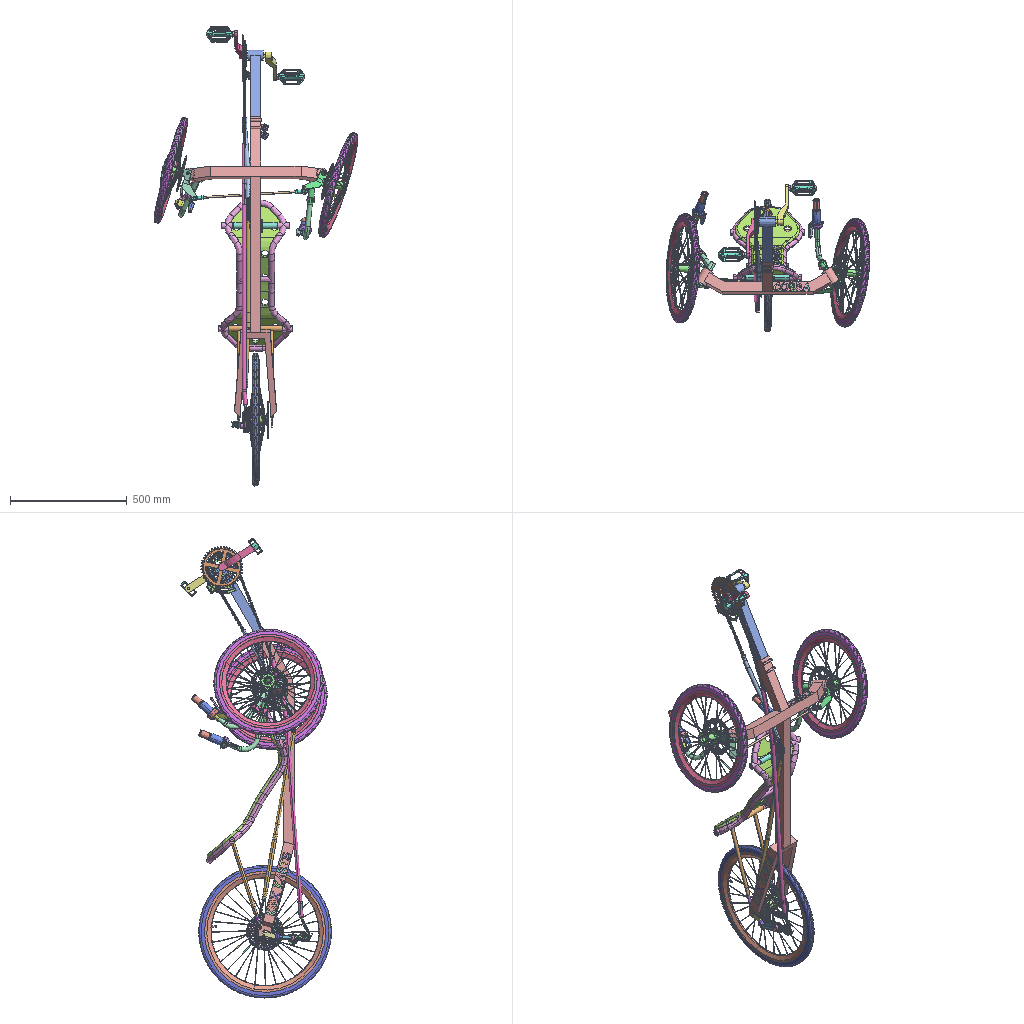Assembly | STEP file | 85 different items | 198 placed | box 873 x 646 x 1971 mm
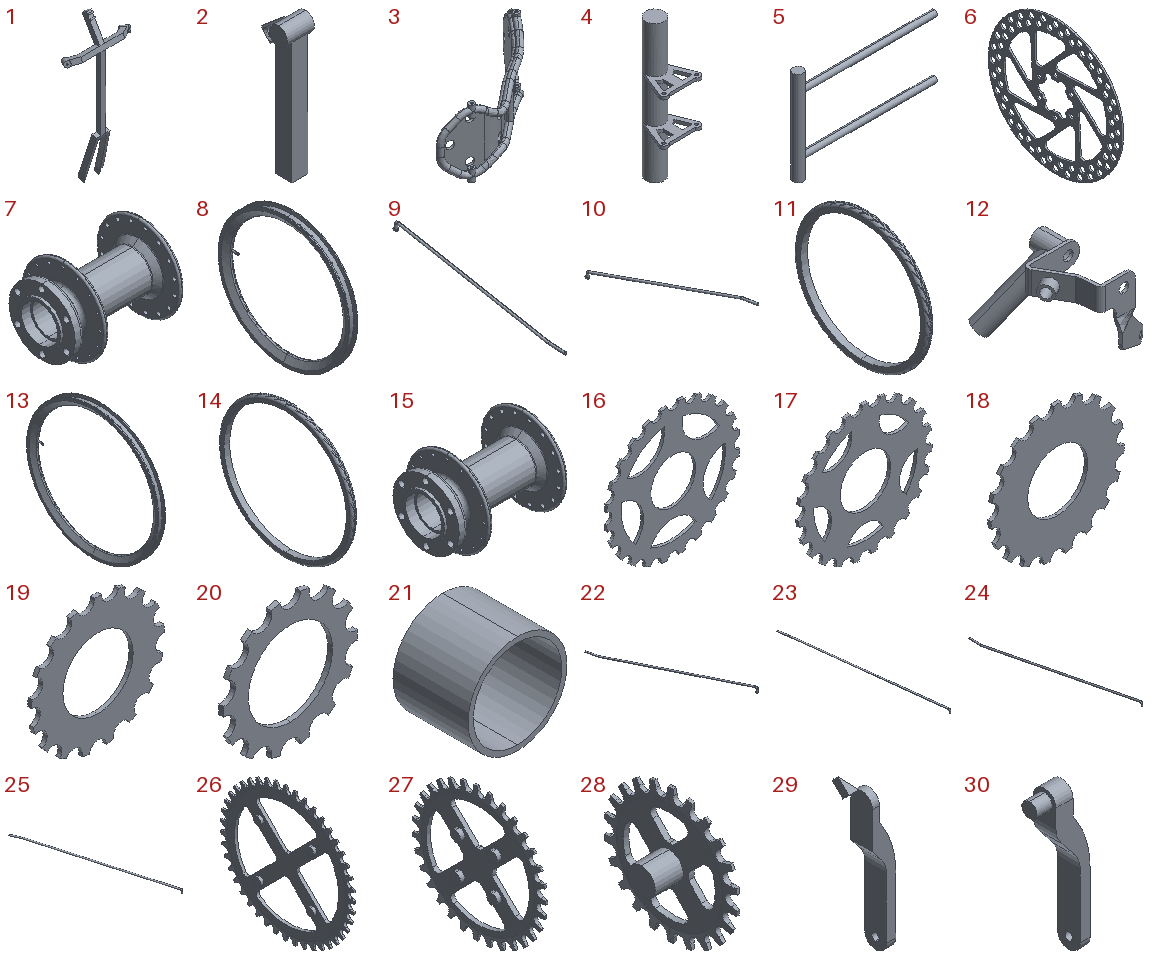Parts list (item | name | quantity | parent item | size | volume):
1 | Cobra Frame | x1 | in Cobra Assembly | 616.506 x 173.118 x 1330 mm | 4060018 mm3
2 | Boom | x1 | in Cobra Assembly | 68 x 96.123 x 337.5 mm | 596645 mm3
3 | Frame | x1 | in KMX_Seat MK10 | 624.751 x 380.553 x 318.558 mm | 2183546 mm3
4 | Frame_Brackets | x1 | in KMX_Seat MK10 | 55 x 52.5 x 189.816 mm | 101287 mm3
5 | Rear_Bar | x1 | in KMX_Seat MK10 | 343.5 x 25 x 228.558 mm | 224969 mm3
6 | Brake Disc | x3 | in KMX Wheel with Disc, Rear Wheel Assembly simple, KMX left Wheel with Disc | 2 x 160 x 160 mm | 16953 mm3
7 | KMX Front Hub | x2 | in KMX Wheel with Disc, KMX left Wheel with Disc | 83.5 x 66 x 66 mm | 47544 mm3
8 | KMX Rim | x2 | in KMX Wheel with Disc, KMX left Wheel with Disc | 30 x 420 x 420 mm | 458838 mm3
9 | Spoke_1 | x32 | in KMX Wheel with Disc, KMX left Wheel with Disc | 8.143 x 171.447 x 36.243 mm | 895.693 mm3
10 | Spoke_IN | x32 | in KMX Wheel with Disc, KMX left Wheel with Disc | 47.785 x 167.549 x 34.429 mm | 896.22 mm3
11 | Royce Quick Tyre | x2 | in KMX Wheel with Disc, KMX left Wheel with Disc | 24 x 468 x 468 mm | 731507 mm3
12 | KMX Cobra Front Pivot RHS | x1 | in Cobra Assembly | 119.015 x 157.368 x 115.563 mm | 46907 mm3
13 | Rear KMX Rim | x1 | in Rear Wheel Assembly simple | 30 x 520 x 520 mm | 578186 mm3
14 | Rear Royce Quick Tyre | x1 | in Rear Wheel Assembly simple | 24 x 568 x 568 mm | 911325 mm3
15 | Rear KMX Hub | x1 | in Rear Wheel Assembly simple | 83.5 x 66 x 66 mm | 47544 mm3
16 | Gear | x1 | in Gear Assembly | 113.111 x 2.2 x 113.111 mm | 12913 mm3
17 | Gear 2 | x1 | in Gear Assembly | 100.969 x 2.2 x 100.781 mm | 10960 mm3
18 | Gear 3 | x1 | in Gear Assembly | 84.766 x 2.2 x 84.54 mm | 8488 mm3
19 | Gear 4 | x1 | in Gear Assembly | 72.249 x 2.2 x 71.994 mm | 5249 mm3
20 | Gear 5 | x1 | in Gear Assembly | 60.7 x 2.2 x 59.972 mm | 2811 mm3
21 | Middle | x1 | in Gear Assembly | 38.2 x 29 x 38.2 mm | 6596 mm3
22 | rear_spoke1 | x8 | in Rear Wheel Assembly simple | 47.236 x 218.366 x 40.79 mm | 731.948 mm3
23 | rear_spoke3 | x8 | in Rear Wheel Assembly simple | 63.794 x 224.344 x 37.5 mm | 749.298 mm3
24 | rear_spoke4 | x8 | in Rear Wheel Assembly simple | 19.566 x 231.981 x 29.396 mm | 746.049 mm3
25 | rear_spoke5 | x8 | in Rear Wheel Assembly simple | 87.859 x 205.125 x 26.5 mm | 711.916 mm3
26 | Front gears | x1 | in Front Crank Assembly | 8 x 179.861 x 179.967 mm | 46199 mm3
27 | Front gears middle | x1 | in Front Crank Assembly | 8 x 129.807 x 129.955 mm | 26124 mm3
28 | Front gears inner | x1 | in Front Crank Assembly | 24 x 95.478 x 96 mm | 23028 mm3
29 | Pedal RHS | x1 | in Front Crank Assembly | 45 x 43.067 x 213.067 mm | 82900 mm3
30 | Pedal LHS | x1 | in Front Crank Assembly | 65 x 30 x 200 mm | 107612 mm3
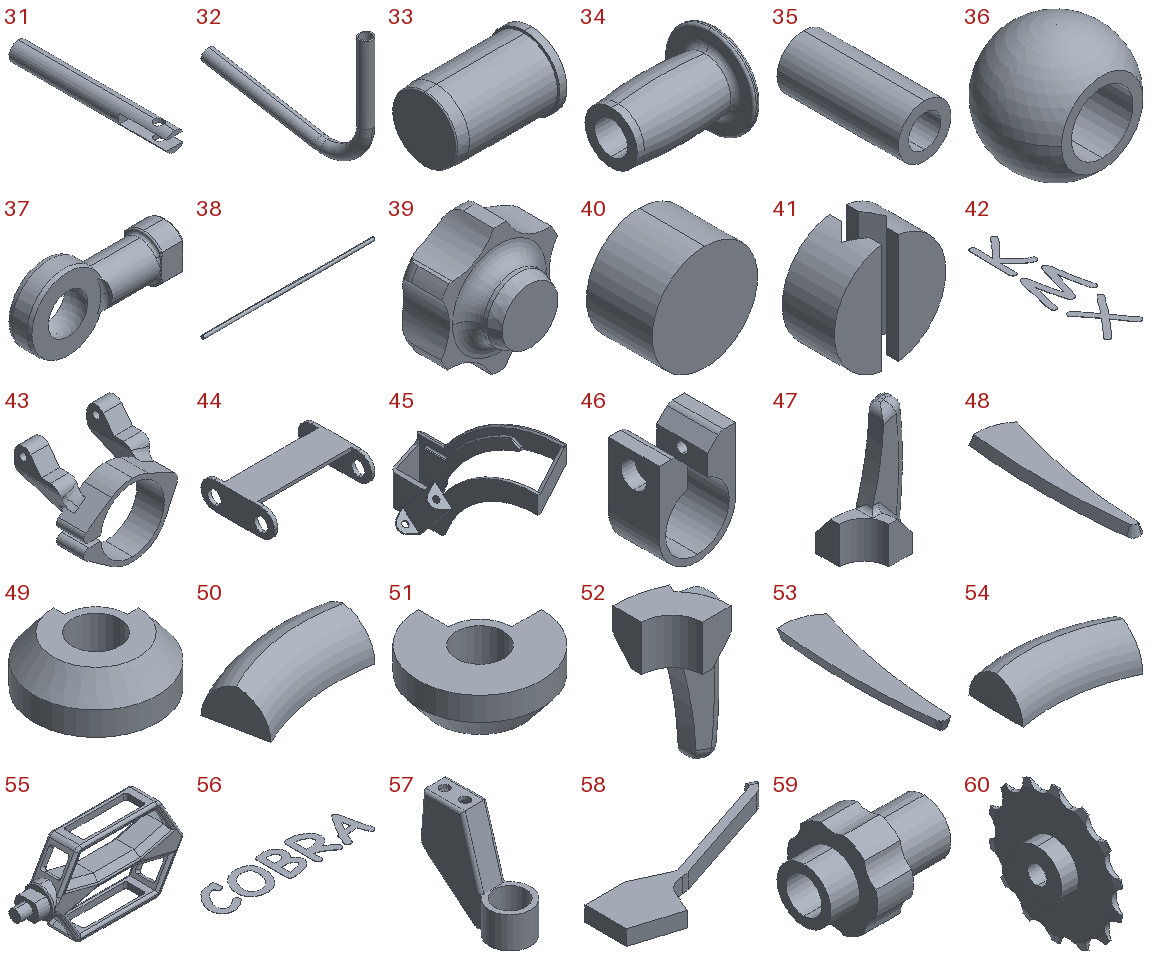31 | Seat Rear Stay | x2 | in Cobra Assembly | 12 x 100 x 12 mm | 9085 mm3
32 | Handlebar | x2 | in Handlebar sub addembly | 20 x 257.938 x 188.495 mm | 45432 mm3
33 | Handlebar end grip | x2 | in Handlebar sub addembly | 45 x 30 x 30 mm | 14675 mm3
34 | Handlebar gear change grip | x2 | in Handlebar sub addembly | 64 x 55 x 55 mm | 44472 mm3
35 | Ball joint spacer | x2 | in Cobra Assembly | 13 x 30 x 13 mm | 2474 mm3
36 | M8 Ball | x2 | in Cobra Assembly | 16 x 12 x 16 mm | 1357 mm3
37 | M8 Body Female | x2 | in Cobra Assembly | 51 x 13 x 26 mm | 5699 mm3
38 | Tie bar | x1 | in Cobra Assembly | 415 x 8 x 8 mm | 20860 mm3
39 | Boom Knob Head | x2 | in Boom Knob | 30.33 x 20 x 33 mm | 9480 mm3
40 | Boom Knob Shaft | x2 | in Boom Knob | 8 x 5 x 8 mm | 251.327 mm3
41 | Shark Fin Adapter | x1 | in Cobra Assembly | 32 x 15 x 31.607 mm | 8681 mm3
42 | KMX Label | x1 | in Cobra Assembly | 37.188 x 122.835 x 0.2 mm | 278.428 mm3
43 | Mounting Bracket v2 | x1 | in Front Derailleur Assembly v2 | 51.858 x 40 x 50 mm | 13111 mm3
44 | Pivot Arm v2 | x1 | in Front Derailleur Assembly v2 | 30 x 22 x 8 mm | 555.338 mm3
45 | Blade v2 | x1 | in Front Derailleur Assembly v2 | 30 x 100.889 x 83.611 mm | 9239 mm3
46 | Handlebar Clamp | x2 | in Cobra Assembly | 30 x 20 x 40 mm | 8999 mm3
47 | Twistshift IndicatorMirror 3 speed | x1 | in TwistGrip 3 Speed Assembly | 33.672 x 26 x 65.01 mm | 13907 mm3
48 | Twistgrip Indicator LensMirror 3 speed | x1 | in TwistGrip 3 Speed Assembly | 12.929 x 50.6 x 3 mm | 990.218 mm3
49 | Twistshift Body3 speed | x1 | in TwistGrip 3 Speed Assembly | 52 x 52 x 20 mm | 23974 mm3
50 | Twistgrip Indicator Line 3 speed | x1 | in TwistGrip 3 Speed Assembly | 6.882 x 4.262 x 1.965 mm | 31.449 mm3
51 | Twistshift Body | x1 | in TwistGrip 9 Speed Assembly | 52 x 52 x 20 mm | 23974 mm3
52 | Twistshift Indicator | x1 | in TwistGrip 9 Speed Assembly | 33.672 x 26 x 65.01 mm | 13907 mm3
53 | Twistgrip Indicator Lens | x1 | in TwistGrip 9 Speed Assembly | 12.929 x 50.6 x 3 mm | 990.218 mm3
54 | Twistgrip Indicator Line | x1 | in TwistGrip 9 Speed Assembly | 6.882 x 4.262 x 1.965 mm | 31.449 mm3
55 | Pedal Basic | x2 | in Cobra Assembly | 131 x 25 x 70 mm | 58244 mm3
56 | Cobra sign | x1 | in Cobra Assembly | 155.556 x 37.16 x 0.2 mm | 521.98 mm3
57 | Dual Brake Lever Body | x1 | in Dual Brake Lever Assembly | 26 x 62.825 x 60 mm | 18209 mm3
58 | Dual Brake Lever Arm | x1 | in Dual Brake Lever Assembly | 101.987 x 44.103 x 8 mm | 8520 mm3
59 | Dual Brake Lever Cable Adjuster | x2 | in Dual Brake Lever Assembly | 13.365 x 10 x 9.679 mm | 483.226 mm3
60 | Metal teeth for metal toothed Idler | x1 | in Metal Toothed Idler | 16 x 56.186 x 57 mm | 8251 mm3
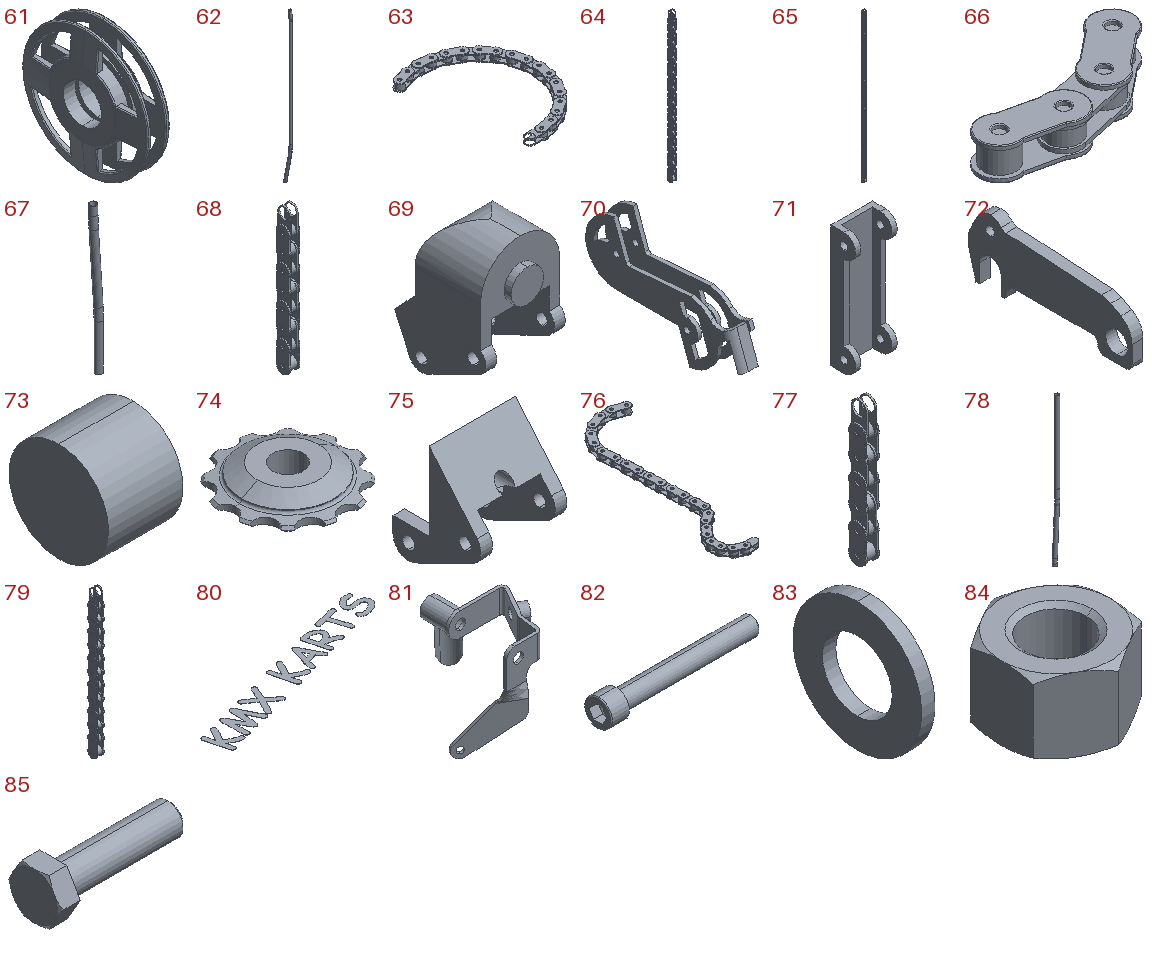61 | Plastic cage for metal toothed Idler | x1 | in Metal Toothed Idler | 15 x 69 x 69 mm | 18640 mm3
62 | Lower Chain Tube | x1 | in Cobra Assembly | 23.853 x 58.527 x 1125 mm | 60168 mm3
63 | Front Crank Chain v2 | x1 | in Cobra Assembly | 94.978 x 131.686 x 8 mm | 9964 mm3
64 | 10 Chain Links v2 | x1 | in Cobra Assembly | 8 x 10 x 280.1 mm | 12161 mm3
65 | 17 Chain Links v2 | x1 | in Cobra Assembly | 8 x 10 x 452.3 mm | 19900 mm3
66 | Idler Chain v2 | x1 | in Cobra Assembly | 45.864 x 21.107 x 8 mm | 2108 mm3
67 | Upper Chain Tube | x1 | in Cobra Assembly | 32.75 x 18 x 400 mm | 21388 mm3
68 | 4 Chain Links v2 | x1 | in Cobra Assembly | 8 x 10 x 107.9 mm | 4422 mm3
69 | Deraillieur Bracket End | x1 | in Cobra Assembly | 22 x 25.773 x 35.5 mm | 7338 mm3
70 | Deraillieur Cage | x1 | in Cobra Assembly | 15 x 100.766 x 59.814 mm | 9684 mm3
71 | Deraillieur Link Arms | x2 | in Cobra Assembly | 16 x 9.5 x 47 mm | 2266 mm3
72 | Deraillieur Mount Brkt | x1 | in Cobra Assembly | 5 x 74.673 x 29.884 mm | 6738 mm3
73 | Deraillieur Mounting spacer | x1 | in Cobra Assembly | 15 x 20 x 20 mm | 4712 mm3
74 | Deraillieur Wheel | x2 | in Cobra Assembly | 39.286 x 39.286 x 10 mm | 5894 mm3
75 | DeraillieurCage End | x1 | in Cobra Assembly | 22 x 22.387 x 28 mm | 2435 mm3
76 | Gear & derail Chain v2 | x1 | in Cobra Assembly | 101.112 x 233.136 x 8 mm | 13651 mm3
77 | 3 Chain Links v2 | x2 | in Cobra Assembly | 8 x 10 x 83.3 mm | 3317 mm3
78 | Rear Chain Tube | x1 | in Cobra Assembly | 29.277 x 18 x 727.809 mm | 34807 mm3
79 | 6 Chain Links v2 | x1 | in Cobra Assembly | 8 x 10 x 157.1 mm | 6633 mm3
80 | KMX KART text | x2 | in Cobra Assembly | 273.592 x 103.676 x 0.2 mm | 837.062 mm3
81 | KMX Cobra Front Pivot LHS | x1 | in left_wheel_assy | 119.015 x 157.368 x 115.563 mm | 46907 mm3
82 | socket head cap screw_bsi_BS EN ISO 4762 M12 x 90 - 36N | x1 | in left_wheel_assy | 102 x 18 x 18 mm | 12605 mm3
83 | plain washer form a_bsi_Bright washer BS 4320 - M12 (Form A) | x2 | in left_wheel_assy | 2.5 x 24 x 24 mm | 799.143 mm3
84 | hex nut gradec_bsi_BS EN 24034 - M12 - N | x2 | in left_wheel_assy | 18 x 20.785 x 12.2 mm | 2394 mm3
85 | hex bolt gradeb_bsi_BS EN 24015 - M12 x 45 x 30-N | x1 | in left_wheel_assy | 52.5 x 20.785 x 18 mm | 7171 mm3
Placements (level | parent | child | x y z in mm | rotation matrix by rows):
1 | Cobra Assembly | Cobra Frame | -9.271 -52.227 425.711 | 1 0 0 0 1 0 0 0 1
1 | Cobra Assembly | Boom | -9.271 152.599 790.593 | 1 0 0 0 0.866 0.5 0 -0.5 0.866
1 | Cobra Assembly | KMX_Seat MK10 | 23.275 145.036 -484.839 | 0 -1e-06 1 -0.0128 0.9999 1e-06 -0.9999 -0.0128 -0
2 | KMX_Seat MK10 | Frame | -451.185 -217.34 -32.545 | 0.9976 0.06944 0 -0.06944 0.9976 -1e-06 0 1e-06 1
2 | KMX_Seat MK10 | Frame_Brackets | -680.581 -160.785 -7.193 | 0.9999 -0.0128 0 0.0128 0.9999 -1e-06 0 1e-06 1
2 | KMX_Seat MK10 | Rear_Bar | -507.128 -158.284 -146.824 | 0.9547 0.2975 0 -0.2975 0.9547 -2e-06 0 2e-06 1
1 | Cobra Assembly | KMX Wheel with Disc | -406.109 23.989 410.865 | -0.9637 0.218 0.1539 0.04863 -0.4236 0.9045 0.2623 0.8792 0.3977
2 | KMX Wheel with Disc | Brake Disc | -74.613 25.526 22.03 | 1 0 0 0 1 0 0 0 1
2 | KMX Wheel with Disc | KMX Front Hub | -26.113 25.526 22.03 | 1 0 0 0 1 -0.007989 0 0.007989 1
2 | KMX Wheel with Disc | KMX Rim | -26.113 25.526 22.03 | 1 0 0 0 1 0 0 0 1
2 | KMX Wheel with Disc | Spoke_1 | 4.887 25.526 22.03 | 0 0 1 0.007989 1 0 -1 0.007989 0
2 | KMX Wheel with Disc | Spoke_IN | 1.887 25.573 21.803 | 0 0 -1 0 1 0 1 0 0
2 | KMX Wheel with Disc | Spoke_1 | 4.887 25.526 22.03 | 0 0 1 0.7127 0.7014 0 -0.7014 0.7127 0
2 | KMX Wheel with Disc | Spoke_1 | 4.887 25.526 22.03 | 0 0 1 1 -0.007989 0 0.007989 1 0
2 | KMX Wheel with Disc | Spoke_1 | 4.887 25.526 22.03 | 0 0 1 0.7014 -0.7127 0 0.7127 0.7014 0
2 | KMX Wheel with Disc | Spoke_1 | 4.887 25.526 22.03 | 0 0 1 -0.007989 -1 0 1 -0.007989 0
2 | KMX Wheel with Disc | Spoke_1 | 4.887 25.526 22.03 | 0 0 1 -0.7127 -0.7014 0 0.7014 -0.7127 0
2 | KMX Wheel with Disc | Spoke_1 | 4.887 25.526 22.03 | 0 0 1 -1 0.007989 0 -0.007989 -1 0
2 | KMX Wheel with Disc | Spoke_1 | 4.887 25.526 22.03 | 0 0 1 -0.7014 0.7127 0 -0.7127 -0.7014 0
2 | KMX Wheel with Disc | Spoke_IN | 1.887 25.72 21.902 | 0 0 -1 -0.7071 0.7071 0 0.7071 0.7071 0
2 | KMX Wheel with Disc | Spoke_IN | 1.887 25.753 22.076 | 0 0 -1 -1 0 0 0 1 0
2 | KMX Wheel with Disc | Spoke_IN | 1.887 25.654 22.223 | 0 0 -1 -0.7071 -0.7071 0 -0.7071 0.7071 0
2 | KMX Wheel with Disc | Spoke_IN | 1.887 25.48 22.257 | 0 0 -1 0 -1 0 -1 0 0
2 | KMX Wheel with Disc | Spoke_IN | 1.887 25.333 22.158 | 0 0 -1 0.7071 -0.7071 0 -0.7071 -0.7071 0
2 | KMX Wheel with Disc | Spoke_IN | 1.887 25.299 21.984 | 0 0 -1 1 0 0 0 -1 0
2 | KMX Wheel with Disc | Spoke_IN | 1.887 25.398 21.837 | 0 0 -1 0.7071 0.7071 0 0.7071 -0.7071 0
2 | KMX Wheel with Disc | Spoke_1 | -57.113 19.465 23.746 | 0 0 -1 -0.9347 0.3555 0 0.3555 0.9347 0
2 | KMX Wheel with Disc | Spoke_IN | -54.113 52.327 4.654 | 0 0 1 0.5718 0.8204 0 -0.8204 0.5718 0
2 | KMX Wheel with Disc | Spoke_IN | -54.113 32.191 -9.207 | 0 0 1 -0.1757 0.9844 0 -0.9844 -0.1757 -0
2 | KMX Wheel with Disc | Spoke_IN | -54.113 8.151 -4.771 | 0 0 1 -0.8204 0.5718 0 -0.5718 -0.8204 -0
2 | KMX Wheel with Disc | Spoke_IN | -54.113 -5.711 15.366 | 0 0 1 -0.9844 -0.1757 0 0.1757 -0.9844 -0
2 | KMX Wheel with Disc | Spoke_IN | -54.113 -1.274 39.405 | 0 0 1 -0.5718 -0.8204 0 0.8204 -0.5718 -0
2 | KMX Wheel with Disc | Spoke_IN | -54.113 18.862 53.267 | 0 0 1 0.1757 -0.9844 0 0.9844 0.1757 -0
2 | KMX Wheel with Disc | Spoke_IN | -54.113 42.902 48.83 | 0 0 1 0.8204 -0.5718 0 0.5718 0.8204 -0
2 | KMX Wheel with Disc | Spoke_IN | -54.113 56.764 28.694 | 0 0 1 0.9844 0.1757 0 -0.1757 0.9844 -0
2 | KMX Wheel with Disc | Spoke_1 | -57.113 22.454 27.529 | 0 0 -1 -0.4096 0.9123 0 0.9123 0.4096 0
2 | KMX Wheel with Disc | Spoke_1 | -57.113 27.242 28.091 | 0 0 -1 0.3555 0.9347 0 0.9347 -0.3555 0
2 | KMX Wheel with Disc | Spoke_1 | -57.113 31.026 25.102 | 0 0 -1 0.9123 0.4096 0 0.4096 -0.9123 0
2 | KMX Wheel with Disc | Spoke_1 | -57.113 31.588 20.314 | 0 0 -1 0.9347 -0.3555 0 -0.3555 -0.9347 0
2 | KMX Wheel with Disc | Spoke_1 | -57.113 28.599 16.53 | 0 0 -1 0.4096 -0.9123 0 -0.9123 -0.4096 0
2 | KMX Wheel with Disc | Spoke_1 | -57.113 23.811 15.968 | 0 0 -1 -0.3555 -0.9347 0 -0.9347 0.3555 0
2 | KMX Wheel with Disc | Spoke_1 | -57.113 20.027 18.957 | 0 0 -1 -0.9123 -0.4096 0 -0.4096 0.9123 0
2 | KMX Wheel with Disc | Royce Quick Tyre | -26.113 25.526 22.03 | 1 0 0 0 0.9997 -0.0264 0 0.0264 0.9997
1 | Cobra Assembly | KMX Cobra Front Pivot RHS | -267.96 3.083 409.302 | 0.8242 0.5 0.266 -0.5391 0.8365 0.09797 -0.1735 -0.2241 0.959
1 | Cobra Assembly | Rear Wheel Assembly simple | -41.175 32.567 -627.976 | -1 0 0 0 0.982 0.1889 0 0.1889 -0.982
2 | Rear Wheel Assembly simple | Rear KMX Rim | -31.903 12.281 8.143 | 1 0 0 0 1 0 0 0 1
2 | Rear Wheel Assembly simple | Rear Royce Quick Tyre | -31.903 12.281 8.143 | 1 0 0 0 1 0 0 0 1
2 | Rear Wheel Assembly simple | Brake Disc | -85.903 12.281 8.143 | 1 0 0 0 -0.8199 0.5725 0 -0.5725 -0.8199
2 | Rear Wheel Assembly simple | Rear KMX Hub | -37.403 12.281 8.143 | 1 0 0 0 -0.8153 0.579 0 -0.579 -0.8153
2 | Rear Wheel Assembly simple | Gear Assembly | -0.2694 7.029 -60.766 | 0 -1 0 0.3818 0 0.9242 -0.9242 0 0.3818
3 | Gear Assembly | Gear | -61.681 0.9337 31.167 | 1 0 0 0 1 0 0 0 1
3 | Gear Assembly | Gear 2 | -61.681 -5.766 31.167 | 0.6463 0 -0.7631 0 1 0 0.7631 0 0.6463
3 | Gear Assembly | Gear 3 | -61.681 -12.466 31.167 | 1 0 0 0 1 0 0 0 1
3 | Gear Assembly | Gear 4 | -61.681 -19.166 31.167 | 1 0 0 0 1 0 0 0 1
3 | Gear Assembly | Gear 5 | -61.681 -25.866 31.167 | 1 0 0 0 1 0 0 0 1
3 | Gear Assembly | Middle | -61.681 -25.866 31.167 | 1 0 0 0 1 0 0 0 1
2 | Rear Wheel Assembly simple | rear_spoke1 | -9.403 12.281 8.143 | 0 0 -1 0.579 -0.8153 0 -0.8153 -0.579 0
2 | Rear Wheel Assembly simple | rear_spoke1 | -9.403 12.281 8.143 | 0 0 -1 -0.1671 -0.9859 0 -0.9859 0.1671 0
2 | Rear Wheel Assembly simple | rear_spoke1 | -9.403 12.281 8.143 | 0 0 -1 -0.8153 -0.579 0 -0.579 0.8153 0
2 | Rear Wheel Assembly simple | rear_spoke1 | -9.403 12.281 8.143 | 0 0 -1 -0.9859 0.1671 0 0.1671 0.9859 0
2 | Rear Wheel Assembly simple | rear_spoke1 | -9.403 12.281 8.143 | 0 0 -1 -0.579 0.8153 0 0.8153 0.579 0
2 | Rear Wheel Assembly simple | rear_spoke1 | -9.403 12.281 8.143 | 0 0 -1 0.1671 0.9859 0 0.9859 -0.1671 0
2 | Rear Wheel Assembly simple | rear_spoke1 | -9.403 12.281 8.143 | 0 0 -1 0.8153 0.579 0 0.579 -0.8153 0
2 | Rear Wheel Assembly simple | rear_spoke1 | -9.403 12.281 8.143 | 0 0 -1 0.9859 -0.1671 0 -0.1671 -0.9859 0
2 | Rear Wheel Assembly simple | rear_spoke3 | -65.403 12.281 8.143 | 0 0 1 -0.579 -0.8153 0 0.8153 -0.579 -0
2 | Rear Wheel Assembly simple | rear_spoke4 | -6.403 12.281 8.143 | 0 0 1 -0.579 -0.8153 0 0.8153 -0.579 -0
2 | Rear Wheel Assembly simple | rear_spoke5 | -9.403 12.281 8.143 | 0 0 -1 0.579 -0.8153 0 -0.8153 -0.579 0
2 | Rear Wheel Assembly simple | rear_spoke3 | -65.403 12.281 8.143 | 0 0 1 0.1671 -0.9859 0 0.9859 0.1671 -0
2 | Rear Wheel Assembly simple | rear_spoke3 | -65.403 12.281 8.143 | 0 0 1 0.8153 -0.579 0 0.579 0.8153 -0
2 | Rear Wheel Assembly simple | rear_spoke3 | -65.403 12.281 8.143 | 0 0 1 0.9859 0.1671 0 -0.1671 0.9859 -0
2 | Rear Wheel Assembly simple | rear_spoke3 | -65.403 12.281 8.143 | 0 0 1 0.579 0.8153 0 -0.8153 0.579 -0
2 | Rear Wheel Assembly simple | rear_spoke3 | -65.403 12.281 8.143 | 0 0 1 -0.1671 0.9859 0 -0.9859 -0.1671 -0
2 | Rear Wheel Assembly simple | rear_spoke3 | -65.403 12.281 8.143 | 0 0 1 -0.8153 0.579 0 -0.579 -0.8153 -0
2 | Rear Wheel Assembly simple | rear_spoke3 | -65.403 12.281 8.143 | 0 0 1 -0.9859 -0.1671 0 0.1671 -0.9859 -0
2 | Rear Wheel Assembly simple | rear_spoke4 | -6.403 12.281 8.143 | 0 0 1 0.1671 -0.9859 0 0.9859 0.1671 -0
2 | Rear Wheel Assembly simple | rear_spoke4 | -6.403 12.281 8.143 | 0 0 1 0.8153 -0.579 0 0.579 0.8153 -0
2 | Rear Wheel Assembly simple | rear_spoke4 | -6.403 12.281 8.143 | 0 0 1 0.9859 0.1671 0 -0.1671 0.9859 -0
2 | Rear Wheel Assembly simple | rear_spoke4 | -6.403 12.281 8.143 | 0 0 1 0.579 0.8153 0 -0.8153 0.579 -0
2 | Rear Wheel Assembly simple | rear_spoke4 | -6.403 12.281 8.143 | 0 0 1 -0.1671 0.9859 0 -0.9859 -0.1671 -0
2 | Rear Wheel Assembly simple | rear_spoke4 | -6.403 12.281 8.143 | 0 0 1 -0.8153 0.579 0 -0.579 -0.8153 -0
2 | Rear Wheel Assembly simple | rear_spoke4 | -6.403 12.281 8.143 | 0 0 1 -0.9859 -0.1671 0 0.1671 -0.9859 -0
2 | Rear Wheel Assembly simple | rear_spoke5 | -9.403 12.281 8.143 | 0 0 -1 -0.1671 -0.9859 0 -0.9859 0.1671 0
2 | Rear Wheel Assembly simple | rear_spoke5 | -9.403 12.281 8.143 | 0 0 -1 -0.8153 -0.579 0 -0.579 0.8153 0
2 | Rear Wheel Assembly simple | rear_spoke5 | -9.403 12.281 8.143 | 0 0 -1 -0.9859 0.1671 0 0.1671 0.9859 0
2 | Rear Wheel Assembly simple | rear_spoke5 | -9.403 12.281 8.143 | 0 0 -1 -0.579 0.8153 0 0.8153 0.579 0
2 | Rear Wheel Assembly simple | rear_spoke5 | -9.403 12.281 8.143 | 0 0 -1 0.1671 0.9859 0 0.9859 -0.1671 0
2 | Rear Wheel Assembly simple | rear_spoke5 | -9.403 12.281 8.143 | 0 0 -1 0.8153 0.579 0 0.579 -0.8153 0
2 | Rear Wheel Assembly simple | rear_spoke5 | -9.403 12.281 8.143 | 0 0 -1 0.9859 -0.1671 0 -0.1671 -0.9859 0
1 | Cobra Assembly | Front Crank Assembly | -67.449 229.667 905.375 | -1 0 0 0 0.5381 0.8429 0 0.8429 -0.5381
2 | Front Crank Assembly | Front gears | -3.178 19.126 -10.215 | 1 0 0 0 1 0 0 0 1
2 | Front Crank Assembly | Front gears middle | -11.178 19.126 -10.215 | 1 0 0 0 1 0 0 0 1
2 | Front Crank Assembly | Front gears inner | -19.178 19.126 -10.215 | 1 0 0 0 1 0 0 0 1
2 | Front Crank Assembly | Pedal RHS | 31.322 19.126 -10.215 | 1 0 0 0 1 0 0 0 1
2 | Front Crank Assembly | Pedal LHS | -147.678 19.126 -10.215 | -1 0 0 0 1 0 0 0 -1
1 | Cobra Assembly | Seat Rear Stay | 60.282 64.68 -621.84 | 0 0 -1 -0.9509 0.3096 0 0.3096 0.9509 0
1 | Cobra Assembly | Seat Rear Stay | -78.825 64.68 -621.84 | 0 0 1 0.9509 0.3096 0 -0.3096 0.9509 0
1 | Cobra Assembly | Handlebar sub addembly | 235.63 187.701 229.027 | 0.9933 -0.04624 0.1059 0.06681 0.9776 -0.1997 -0.09429 0.2055 0.9741
2 | Handlebar sub addembly | Handlebar | -25.887 -114.099 104.599 | 1 0 0 0 1 0 0 0 1
2 | Handlebar sub addembly | Handlebar end grip | -25.887 135.057 -41.468 | 0 0.9848 0.1736 -0.9848 0.03015 -0.171 -0.1736 -0.171 0.9698
2 | Handlebar sub addembly | Handlebar gear change grip | -25.887 90.741 -49.282 | 0 0.2701 0.9628 -0.9848 0.1672 -0.0469 -0.1736 -0.9482 0.266
1 | Cobra Assembly | Handlebar sub addembly | -265.415 217.618 325.837 | 0.9126 0.1973 0.3582 0.02626 0.8459 -0.5327 -0.4081 0.4955 0.7667
2 | Handlebar sub addembly | Handlebar | -25.887 -114.099 104.599 | 1 0 0 0 1 0 0 0 1
2 | Handlebar sub addembly | Handlebar end grip | -25.887 135.057 -41.468 | 0 0.9848 0.1736 -0.9848 0.03015 -0.171 -0.1736 -0.171 0.9698
2 | Handlebar sub addembly | Handlebar gear change grip | -25.887 90.741 -49.282 | 0 0.2701 0.9628 -0.9848 0.1672 -0.0469 -0.1736 -0.9482 0.266
1 | Cobra Assembly | Ball joint spacer | -270.273 -18.938 317.235 | 0.1139 -0.02093 -0.9933 -0.109 -0.994 0.008443 -0.9875 0.1074 -0.1155
1 | Cobra Assembly | Ball joint spacer | 199.528 -43.232 347.474 | -0.4628 0.0305 -0.8859 -0.3961 -0.9012 0.1759 -0.793 0.4323 0.4292
1 | Cobra Assembly | M8 Ball | -270.049 -8.312 316.088 | -0.7903 -0.02093 -0.6123 -0.04931 -0.994 0.09763 -0.6107 0.1074 0.7846
1 | Cobra Assembly | M8 Ball | 199.202 -33.598 342.853 | -0.996 0.0305 -0.08359 -0.06357 -0.9012 0.4287 -0.06226 0.4323 0.8996
1 | Cobra Assembly | M8 Body Female | -270.147 -12.974 316.591 | 0.9968 0.06348 -0.0486 -0.05276 0.9791 0.1966 0.06006 -0.1934 0.9793
1 | Cobra Assembly | M8 Body Female | 199.345 -37.825 344.88 | -0.9968 -0.05678 -0.05628 0.05276 -0.9961 0.07046 -0.06006 0.06726 0.9959
1 | Cobra Assembly | Tie bar | -35.401 -25.399 330.736 | 0.9968 -0.07848 0.01523 -0.05276 -0.789 -0.6122 0.06006 0.6094 -0.7906
1 | Cobra Assembly | Boom Knob | 10.136 76.512 609.256 | 0.6899 0.7071 0.1551 -0.7071 0.6124 0.3536 0.1551 -0.3536 0.9225
2 | Boom Knob | Boom Knob Head | 8.251 11.809 -19.171 | 1 0 0 0 1 0 0 0 1
2 | Boom Knob | Boom Knob Shaft | 8.251 6.809 -19.171 | 0.995 0 0.0996 0 1 0 -0.0996 0 0.995
1 | Cobra Assembly | Boom Knob | 10.136 95.624 642.216 | 0.6899 0.7071 0.1551 -0.7071 0.6124 0.3536 0.1551 -0.3536 0.9225
2 | Boom Knob | Boom Knob Head | 8.251 11.809 -19.171 | 1 0 0 0 1 0 0 0 1
2 | Boom Knob | Boom Knob Shaft | 8.251 6.809 -19.171 | 0.995 0 0.0996 0 1 0 -0.0996 0 0.995
1 | Cobra Assembly | Shark Fin Adapter | -9.271 262.298 861.978 | 1 0 0 0 0.342 0.9397 0 -0.9397 0.342
1 | Cobra Assembly | KMX Label | -9.271 -37.565 417.21 | -1 0 0 0 0.5016 0.8651 0 0.8651 -0.5016
1 | Cobra Assembly | Front Derailleur Assembly v2 | -6.165 280.687 856.044 | 0 0 -1 0.9397 0.342 0 0.342 -0.9397 0
2 | Front Derailleur Assembly v2 | Mounting Bracket v2 | -15.25 -4.365 3.106 | 1 0 0 0 1 0 0 0 1
2 | Front Derailleur Assembly v2 | Pivot Arm v2 | -15.25 19.29 26.405 | 1 0 0 0 0.8473 0.531 0 -0.531 0.8473
2 | Front Derailleur Assembly v2 | Blade v2 | -35.704 -77.471 60.541 | 0 0.6428 -0.766 0 0.766 0.6428 1 0 -0
1 | Cobra Assembly | Handlebar Clamp | -290.197 88.674 325.558 | -0.9126 -0.3582 -0.1973 -0.02626 0.5327 -0.8459 0.4081 -0.7667 -0.4955
1 | Cobra Assembly | Handlebar Clamp | 226.482 53.141 311.863 | -0.9933 -0.1059 0.04624 -0.06681 0.1997 -0.9776 0.09429 -0.9741 -0.2055
1 | Cobra Assembly | TwistGrip 3 Speed Assembly | 225.556 192.252 139.431 | -0.7981 -0.6019 0.02715 -0.2439 0.2815 -0.928 0.5509 -0.7473 -0.3715
2 | TwistGrip 3 Speed Assembly | Twistshift IndicatorMirror 3 speed | 32.023 -5.779 -45.592 | 1 0 0 0 1 0 0 0 1
2 | TwistGrip 3 Speed Assembly | Twistgrip Indicator LensMirror 3 speed | 32.023 11.221 -45.592 | -1 0 0 0 0 -1 0 -1 0
2 | TwistGrip 3 Speed Assembly | Twistshift Body3 speed | 32.023 -5.779 -45.592 | 1 0 0 0 1 0 0 0 1
2 | TwistGrip 3 Speed Assembly | Twistgrip Indicator Line 3 speed | 32.023 11.221 -45.592 | 1 0 0 0 0 1 0 -1 0
1 | Cobra Assembly | TwistGrip 9 Speed Assembly | -316.977 273.079 310.249 | 0.8856 0.3872 0.2565 -0.4375 0.5101 0.7405 0.1559 -0.768 0.6212
2 | TwistGrip 9 Speed Assembly | Twistshift Body | 9.652 9.221 -1.358 | 1 0 0 0 1 0 0 0 1
2 | TwistGrip 9 Speed Assembly | Twistshift Indicator | 9.652 9.221 -1.358 | 1 0 0 0 1 0 0 0 1
2 | TwistGrip 9 Speed Assembly | Twistgrip Indicator Lens | 9.652 26.221 -1.358 | -1 0 0 0 0 1 0 1 0
2 | TwistGrip 9 Speed Assembly | Twistgrip Indicator Line | 9.652 26.221 -1.358 | -1 0 0 0 0 1 0 1 0
1 | Cobra Assembly | Pedal Basic | -164.771 88.06 1018.471 | -1 0 0 0 -0.806 0.5919 0 0.5919 0.806
1 | Cobra Assembly | Pedal Basic | 146.229 374.638 835.514 | 1 0 0 0 -0.6753 -0.7376 0 0.7376 -0.6753
1 | Cobra Assembly | Cobra sign | -9.271 -46.403 447.445 | 1 0 0 0 0.9659 0.2588 0 -0.2588 0.9659
1 | Cobra Assembly | Dual Brake Lever Assembly | -299.341 223.791 299.843 | 0.8119 -0.5245 -0.2565 -0.5138 -0.4332 -0.7405 0.2773 0.733 -0.6212
2 | Dual Brake Lever Assembly | Dual Brake Lever Body | -28.71 -15.127 -17.082 | 1 0 0 0 1 0 0 0 1
2 | Dual Brake Lever Assembly | Dual Brake Lever Arm | -28.71 -15.127 -17.082 | 0 0 1 0 1 0 -1 0 0
2 | Dual Brake Lever Assembly | Dual Brake Lever Cable Adjuster | -28.71 -15.127 -17.082 | 0 0 1 0 1 0 -1 0 0
2 | Dual Brake Lever Assembly | Dual Brake Lever Cable Adjuster | -69.49 22.528 -17.082 | 0 0.9769 -0.2135 0 -0.2135 -0.9769 -1 0 -0
1 | Cobra Assembly | Metal Toothed Idler | 2.952 -65.559 245.75 | 1 0 0 0 1 0 0 0 1
2 | Metal Toothed Idler | Metal teeth for metal toothed Idler | -42.723 8.797 16.568 | 1 0 0 0 1 0 0 0 1
2 | Metal Toothed Idler | Plastic cage for metal toothed Idler | -42.723 8.797 16.568 | 1 0 0 0 1 0 0 0 1
1 | Cobra Assembly | Lower Chain Tube | -58.165 -102.891 -499.513 | -1 0 0 0 0.9971 -0.07653 0 -0.07653 -0.9971
1 | Cobra Assembly | Front Crank Chain v2 | -56.271 231.157 926.813 | 0 0 -1 0.4003 0.9164 0 0.9164 -0.4003 -0
1 | Cobra Assembly | 10 Chain Links v2 | -56.271 141.25 660.093 | 1 0 0 0 0.8604 0.5097 0 -0.5097 0.8604
1 | Cobra Assembly | 17 Chain Links v2 | -56.271 168.641 933.986 | 1 0 0 0 -0.9327 -0.3606 0 0.3606 -0.9327
1 | Cobra Assembly | Idler Chain v2 | -39.771 -56.761 262.318 | 0 0 -1 0 1 0 1 0 0
1 | Cobra Assembly | Upper Chain Tube | -41.521 -10.393 398.649 | 1 0 0 0 0.866 0.5 0 -0.5 0.866
1 | Cobra Assembly | 4 Chain Links v2 | -39.771 -31.27 359.459 | 1 0 0 0 -0.8604 -0.5097 0 0.5097 -0.8604
1 | Cobra Assembly | Deraillieur Bracket End | -88.825 -22.698 -653.863 | 0 -1 0 0.1216 0 0.9926 -0.9926 0 0.1216
1 | Cobra Assembly | Deraillieur Cage | -52.121 -74.863 -669.055 | -1 0 0 0 0.9993 0.03743 0 0.03743 -0.9993
1 | Cobra Assembly | Deraillieur Link Arms | -88.825 -22.698 -653.863 | 0 0.859 -0.512 -0.1216 0.5082 0.8526 0.9926 0.06225 0.1045
1 | Cobra Assembly | Deraillieur Link Arms | -103.212 -29.647 -654.714 | 0 -0.859 -0.512 0.1216 -0.5082 0.8526 -0.9926 -0.06225 0.1045
1 | Cobra Assembly | Deraillieur Mount Brkt | -84.325 46.165 -633.651 | -1 0 0 0 0.9477 0.3191 0 0.3191 -0.9477
1 | Cobra Assembly | Deraillieur Mounting spacer | -74.621 -69.243 -659.565 | 1 0 0 0 0.9993 -0.03632 0 0.03632 0.9993
1 | Cobra Assembly | Deraillieur Wheel | -52.121 -121.405 -650.784 | 0 0 -1 0 1 0 1 0 -0
1 | Cobra Assembly | Deraillieur Wheel | -52.121 -74.863 -669.055 | 0 0 -1 0 1 0 1 0 -0
1 | Cobra Assembly | DeraillieurCage End | -74.621 -69.243 -659.565 | 0 1 0 0.1216 0 -0.9926 -0.9926 0 -0.1216
1 | Cobra Assembly | Gear & derail Chain v2 | -53.371 46.165 -633.651 | 0 0 -1 0.2003 0.9797 0 0.9797 -0.2003 0
1 | Cobra Assembly | 3 Chain Links v2 | -52.271 -114.187 -584.276 | 1 0 0 0 -0.9107 -0.4131 0 0.4131 -0.9107
1 | Cobra Assembly | Rear Chain Tube | -40.771 -75.29 221.587 | 1 0 0 0 0.9848 -0.1736 0 0.1736 0.9848
1 | Cobra Assembly | 3 Chain Links v2 | -39.771 -69.274 189.649 | 1 0 0 0 0.9735 -0.2287 0 0.2287 0.9735
1 | Cobra Assembly | 6 Chain Links v2 | -52.271 50.542 -490.984 | 1 0 0 0 -0.9635 0.2676 0 -0.2676 -0.9635
1 | Cobra Assembly | KMX KART text | 2.106 -52.456 426.567 | 0.075 0.02016 0.997 -0.001512 0.9998 -0.0201 -0.9972 0 0.07501
1 | Cobra Assembly | KMX KART text | -150.474 383.88 -1181.942 | 0.0749 0.02051 -0.997 -0.5039 0.8635 -0.0201 0.8605 0.5039 0.07501
1 | Cobra Assembly | left_wheel_assy | 250.013 3.174 412.775 | 0.805 -0.5 0.3193 0.3535 0.8365 0.4186 -0.4764 -0.2241 0.8502
2 | left_wheel_assy | KMX Cobra Front Pivot LHS | -0.0 -0.0 -0.0 | 1 0 0 0 1 0 0 0 1
2 | left_wheel_assy | socket head cap screw_bsi_BS EN ISO 4762 M12 x 90 - 36N | 5.0 35.414 -0.0 | 0 -0.817 0.5766 -1 0 0 0 -0.5766 -0.817
2 | left_wheel_assy | plain washer form a_bsi_Bright washer BS 4320 - M12 (Form A) | 5.0 -54.586 -0.0 | 0 -0.3786 0.9255 1 0 0 0 0.9255 0.3786
2 | left_wheel_assy | hex nut gradec_bsi_BS EN 24034 - M12 - N | 5.0 -57.086 -0.0 | 0.9239 -0.3826 0 0 0 1 -0.3826 -0.9239 -0
2 | left_wheel_assy | hex bolt gradeb_bsi_BS EN 24015 - M12 x 45 x 30-N | 82.93 -19.27 1.538 | -0.866 0.3548 0.3523 0.5 0.6146 0.6101 0 0.7045 -0.7097
2 | left_wheel_assy | plain washer form a_bsi_Bright washer BS 4320 - M12 (Form A) | 46.817 1.58 1.538 | -0.866 -0.2794 0.4146 0.5 -0.484 0.7182 0 0.8293 0.5589
2 | left_wheel_assy | hex nut gradec_bsi_BS EN 24034 - M12 - N | 36.252 7.68 1.538 | 0.4912 -0.0934 -0.866 0.8508 -0.1618 0.5 -0.1868 -0.9824 0
2 | left_wheel_assy | KMX left Wheel with Disc | 115.762 -54.628 -31.093 | 0.866 0.4477 -0.2227 -0.5 0.7754 -0.3857 0 0.4453 0.8954
3 | KMX left Wheel with Disc | Brake Disc | -74.613 25.526 22.03 | 1 0 0 0 1 0 0 0 1
3 | KMX left Wheel with Disc | KMX Front Hub | -26.113 25.526 22.03 | 1 0 0 0 1 -0.007989 0 0.007989 1
3 | KMX left Wheel with Disc | KMX Rim | -26.113 25.526 22.03 | 1 0 0 0 1 0 0 0 1
3 | KMX left Wheel with Disc | Spoke_1 | 4.887 25.526 22.03 | 0 0 1 0.007989 1 0 -1 0.007989 0
3 | KMX left Wheel with Disc | Spoke_IN | 1.887 25.573 21.803 | 0 0 -1 0 1 0 1 0 -0
3 | KMX left Wheel with Disc | Spoke_1 | 4.887 25.526 22.03 | 0 0 1 0.7127 0.7014 0 -0.7014 0.7127 0
3 | KMX left Wheel with Disc | Spoke_1 | 4.887 25.526 22.03 | 0 0 1 1 -0.007989 0 0.007989 1 0
3 | KMX left Wheel with Disc | Spoke_1 | 4.887 25.526 22.03 | 0 0 1 0.7014 -0.7127 0 0.7127 0.7014 0
3 | KMX left Wheel with Disc | Spoke_1 | 4.887 25.526 22.03 | 0 0 1 -0.007989 -1 0 1 -0.007989 0
3 | KMX left Wheel with Disc | Spoke_1 | 4.887 25.526 22.03 | 0 0 1 -0.7127 -0.7014 0 0.7014 -0.7127 0
3 | KMX left Wheel with Disc | Spoke_1 | 4.887 25.526 22.03 | 0 0 1 -1 0.007989 0 -0.007989 -1 0
3 | KMX left Wheel with Disc | Spoke_1 | 4.887 25.526 22.03 | 0 0 1 -0.7014 0.7127 0 -0.7127 -0.7014 0
3 | KMX left Wheel with Disc | Spoke_IN | 1.887 25.72 21.902 | 0 0 -1 -0.7071 0.7071 0 0.7071 0.7071 -0
3 | KMX left Wheel with Disc | Spoke_IN | 1.887 25.753 22.076 | 0 0 -1 -1 0 0 0 1 -0
3 | KMX left Wheel with Disc | Spoke_IN | 1.887 25.654 22.223 | 0 0 -1 -0.7071 -0.7071 0 -0.7071 0.7071 -0
3 | KMX left Wheel with Disc | Spoke_IN | 1.887 25.48 22.257 | 0 0 -1 0 -1 0 -1 0 -0
3 | KMX left Wheel with Disc | Spoke_IN | 1.887 25.333 22.158 | 0 0 -1 0.7071 -0.7071 0 -0.7071 -0.7071 -0
3 | KMX left Wheel with Disc | Spoke_IN | 1.887 25.299 21.984 | 0 0 -1 1 0 0 0 -1 -0
3 | KMX left Wheel with Disc | Spoke_IN | 1.887 25.398 21.837 | 0 0 -1 0.7071 0.7071 0 0.7071 -0.7071 -0
3 | KMX left Wheel with Disc | Spoke_1 | -57.113 19.465 23.746 | 0 0 -1 -0.9347 0.3555 0 0.3555 0.9347 -0
3 | KMX left Wheel with Disc | Spoke_IN | -54.113 52.327 4.654 | 0 0 1 0.5718 0.8204 0 -0.8204 0.5718 0
3 | KMX left Wheel with Disc | Spoke_IN | -54.113 32.191 -9.207 | 0 0 1 -0.1757 0.9844 0 -0.9844 -0.1757 0
3 | KMX left Wheel with Disc | Spoke_IN | -54.113 8.151 -4.771 | 0 0 1 -0.8204 0.5718 0 -0.5718 -0.8204 0
3 | KMX left Wheel with Disc | Spoke_IN | -54.113 -5.711 15.366 | 0 0 1 -0.9844 -0.1757 0 0.1757 -0.9844 0
3 | KMX left Wheel with Disc | Spoke_IN | -54.113 -1.274 39.405 | 0 0 1 -0.5718 -0.8204 0 0.8204 -0.5718 -0
3 | KMX left Wheel with Disc | Spoke_IN | -54.113 18.862 53.267 | 0 0 1 0.1757 -0.9844 0 0.9844 0.1757 -0
3 | KMX left Wheel with Disc | Spoke_IN | -54.113 42.902 48.83 | 0 0 1 0.8204 -0.5718 0 0.5718 0.8204 0
3 | KMX left Wheel with Disc | Spoke_IN | -54.113 56.764 28.694 | 0 0 1 0.9844 0.1757 0 -0.1757 0.9844 0
3 | KMX left Wheel with Disc | Spoke_1 | -57.113 22.454 27.529 | 0 0 -1 -0.4096 0.9123 0 0.9123 0.4096 -0
3 | KMX left Wheel with Disc | Spoke_1 | -57.113 27.242 28.091 | 0 0 -1 0.3555 0.9347 0 0.9347 -0.3555 -0
3 | KMX left Wheel with Disc | Spoke_1 | -57.113 31.026 25.102 | 0 0 -1 0.9123 0.4096 0 0.4096 -0.9123 0
3 | KMX left Wheel with Disc | Spoke_1 | -57.113 31.588 20.314 | 0 0 -1 0.9347 -0.3555 0 -0.3555 -0.9347 -0
3 | KMX left Wheel with Disc | Spoke_1 | -57.113 28.599 16.53 | 0 0 -1 0.4096 -0.9123 0 -0.9123 -0.4096 0
3 | KMX left Wheel with Disc | Spoke_1 | -57.113 23.811 15.968 | 0 0 -1 -0.3555 -0.9347 0 -0.9347 0.3555 0
3 | KMX left Wheel with Disc | Spoke_1 | -57.113 20.027 18.957 | 0 0 -1 -0.9123 -0.4096 0 -0.4096 0.9123 -0
3 | KMX left Wheel with Disc | Royce Quick Tyre | -26.113 25.526 22.03 | -1 0 0 0 0.3765 -0.9264 0 -0.9264 -0.3765